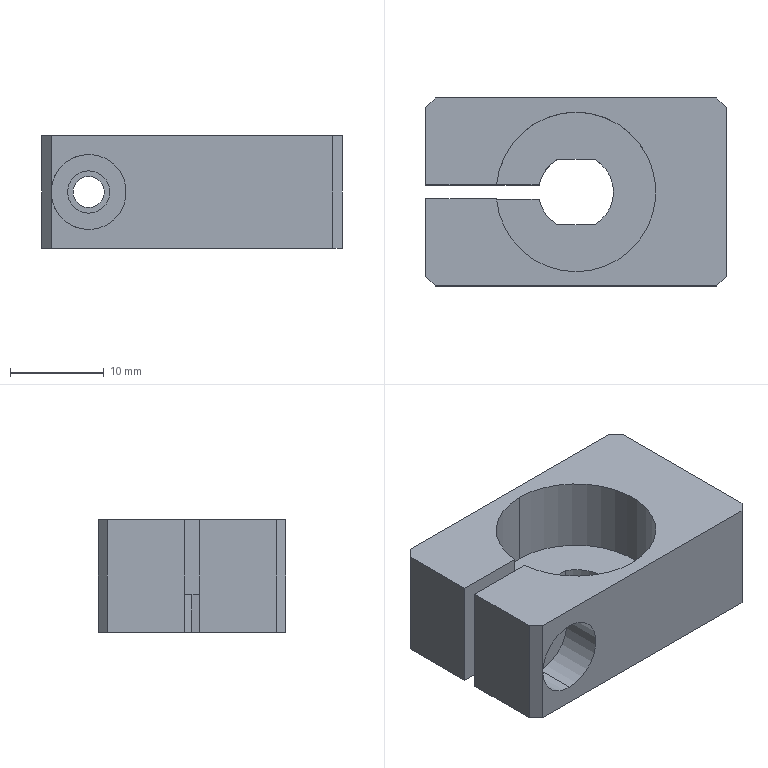Part | SolidWorks | features ICE 3, HoleWzd 2, Chamfer 1, Extrusion 1, RevCut 1 | 1 solid | 30 faces | box 32 x 20 x 12 mm | volume 5110 mm3 | plane 17 | cylinder 13 | commonest cylinder face diameters 8 x6 17 x3 3.3 x2 4.5 x2
STEP:
#1=CARTESIAN_POINT('',(-11.,10.,1.65));
#2=VERTEX_POINT('',#1);
#3=CARTESIAN_POINT('',(-11.,10.,-1.65));
#4=VERTEX_POINT('',#3);
#5=CARTESIAN_POINT('',(-11.,10.,0.));
#6=DIRECTION('',(0.,-1.,0.));
#7=DIRECTION('',(0.,0.,-1.));
#8=AXIS2_PLACEMENT_3D('',#5,#6,#7);
#9=CIRCLE('',#8,1.65);
#10=EDGE_CURVE('',#2,#4,#9,.T.);
#11=ORIENTED_EDGE('',*,*,#10,.F.);
#12=CARTESIAN_POINT('',(-11.,0.75,1.65));
#13=VERTEX_POINT('',#12);
#14=CARTESIAN_POINT('',(-11.,0.75,1.65));
#15=DIRECTION('',(0.,-1.,0.));
#16=VECTOR('',#15,1000.);
#17=LINE('',#14,#16);
#18=EDGE_CURVE('',#2,#13,#17,.T.);
#19=ORIENTED_EDGE('',*,*,#18,.T.);
#20=CARTESIAN_POINT('',(-11.,0.75,-1.65));
#21=VERTEX_POINT('',#20);
#22=CARTESIAN_POINT('',(-11.,0.75,0.));
#23=DIRECTION('',(0.,-1.,0.));
#24=DIRECTION('',(0.,0.,-1.));
#25=AXIS2_PLACEMENT_3D('',#22,#23,#24);
#26=CIRCLE('',#25,1.65);
#27=EDGE_CURVE('',#13,#21,#26,.T.);
#28=ORIENTED_EDGE('',*,*,#27,.T.);
#29=CARTESIAN_POINT('',(-11.,0.75,-1.65));
#30=DIRECTION('',(0.,-1.,0.));
#31=VECTOR('',#30,1000.);
#32=LINE('',#29,#31);
#33=EDGE_CURVE('',#4,#21,#32,.T.);
#34=ORIENTED_EDGE('',*,*,#33,.F.);
#35=EDGE_LOOP('',(#11,#19,#28,#34));
#36=FACE_OUTER_BOUND('',#35,.T.);
#37=CARTESIAN_POINT('',(-11.,0.75,0.));
#38=DIRECTION('',(0.,-1.,0.));
#39=DIRECTION('',(0.,0.,-1.));
#40=AXIS2_PLACEMENT_3D('',#37,#38,#39);
#41=CYLINDRICAL_SURFACE('',#40,1.65);
#42=ADVANCED_FACE('',(#36),#41,.F.);
#43=CARTESIAN_POINT('',(-11.,-5.6,4.));
#44=VERTEX_POINT('',#43);
#45=CARTESIAN_POINT('',(-11.,-5.6,-4.));
#46=VERTEX_POINT('',#45);
#47=CARTESIAN_POINT('',(-11.,-5.6,0.));
#48=DIRECTION('',(0.,-1.,0.));
#49=DIRECTION('',(0.,0.,-1.));
#50=AXIS2_PLACEMENT_3D('',#47,#48,#49);
#51=CIRCLE('',#50,4.);
#52=EDGE_CURVE('',#44,#46,#51,.T.);
#53=ORIENTED_EDGE('',*,*,#52,.F.);
#54=CARTESIAN_POINT('',(-11.,-10.,4.));
#55=VERTEX_POINT('',#54);
#56=CARTESIAN_POINT('',(-11.,-10.,4.));
#57=DIRECTION('',(0.,-1.,0.));
#58=VECTOR('',#57,1000.);
#59=LINE('',#56,#58);
#60=EDGE_CURVE('',#44,#55,#59,.T.);
#61=ORIENTED_EDGE('',*,*,#60,.T.);
#62=CARTESIAN_POINT('',(-15.,-10.,0.));
#63=VERTEX_POINT('',#62);
#64=CARTESIAN_POINT('',(-11.,-10.,0.));
#65=DIRECTION('',(0.,-1.,0.));
#66=DIRECTION('',(0.,0.,-1.));
#67=AXIS2_PLACEMENT_3D('',#64,#65,#66);
#68=CIRCLE('',#67,4.);
#69=EDGE_CURVE('',#55,#63,#68,.T.);
#70=ORIENTED_EDGE('',*,*,#69,.T.);
#71=CARTESIAN_POINT('',(-11.,-10.,-4.));
#72=VERTEX_POINT('',#71);
#73=CARTESIAN_POINT('',(-11.,-10.,0.));
#74=DIRECTION('',(0.,-1.,0.));
#75=DIRECTION('',(0.,0.,-1.));
#76=AXIS2_PLACEMENT_3D('',#73,#74,#75);
#77=CIRCLE('',#76,4.);
#78=EDGE_CURVE('',#63,#72,#77,.T.);
#79=ORIENTED_EDGE('',*,*,#78,.T.);
#80=CARTESIAN_POINT('',(-11.,-10.,-4.));
#81=DIRECTION('',(0.,-1.,0.));
#82=VECTOR('',#81,1000.);
#83=LINE('',#80,#82);
#84=EDGE_CURVE('',#46,#72,#83,.T.);
#85=ORIENTED_EDGE('',*,*,#84,.F.);
#86=EDGE_LOOP('',(#53,#61,#70,#79,#85));
#87=FACE_OUTER_BOUND('',#86,.T.);
#88=CARTESIAN_POINT('',(-11.,-10.,0.));
#89=DIRECTION('',(0.,-1.,0.));
#90=DIRECTION('',(0.,0.,-1.));
#91=AXIS2_PLACEMENT_3D('',#88,#89,#90);
#92=CYLINDRICAL_SURFACE('',#91,4.);
#93=ADVANCED_FACE('',(#87),#92,.F.);
#94=CARTESIAN_POINT('',(-11.,-0.75,2.25));
#95=VERTEX_POINT('',#94);
#96=CARTESIAN_POINT('',(-11.,-0.75,-2.25));
#97=VERTEX_POINT('',#96);
#98=CARTESIAN_POINT('',(-11.,-0.75,0.));
#99=DIRECTION('',(0.,-1.,0.));
#100=DIRECTION('',(0.,0.,-1.));
#101=AXIS2_PLACEMENT_3D('',#98,#99,#100);
#102=CIRCLE('',#101,2.25);
#103=EDGE_CURVE('',#95,#97,#102,.T.);
#104=ORIENTED_EDGE('',*,*,#103,.F.);
#105=CARTESIAN_POINT('',(-11.,-5.6,2.25));
#106=VERTEX_POINT('',#105);
#107=CARTESIAN_POINT('',(-11.,-10.,2.25));
#108=DIRECTION('',(0.,-1.,0.));
#109=VECTOR('',#108,1000.);
#110=LINE('',#107,#109);
#111=EDGE_CURVE('',#95,#106,#110,.T.);
#112=ORIENTED_EDGE('',*,*,#111,.T.);
#113=CARTESIAN_POINT('',(-11.,-5.6,-2.25));
#114=VERTEX_POINT('',#113);
#115=CARTESIAN_POINT('',(-11.,-5.6,0.));
#116=DIRECTION('',(0.,-1.,0.));
#117=DIRECTION('',(0.,0.,-1.));
#118=AXIS2_PLACEMENT_3D('',#115,#116,#117);
#119=CIRCLE('',#118,2.25);
#120=EDGE_CURVE('',#106,#114,#119,.T.);
#121=ORIENTED_EDGE('',*,*,#120,.T.);
#122=CARTESIAN_POINT('',(-11.,-10.,-2.25));
#123=DIRECTION('',(0.,-1.,0.));
#124=VECTOR('',#123,1000.);
#125=LINE('',#122,#124);
#126=EDGE_CURVE('',#97,#114,#125,.T.);
#127=ORIENTED_EDGE('',*,*,#126,.F.);
#128=EDGE_LOOP('',(#104,#112,#121,#127));
#129=FACE_OUTER_BOUND('',#128,.T.);
#130=CARTESIAN_POINT('',(-11.,-10.,0.));
#131=DIRECTION('',(0.,-1.,0.));
#132=DIRECTION('',(0.,0.,-1.));
#133=AXIS2_PLACEMENT_3D('',#130,#131,#132);
#134=CYLINDRICAL_SURFACE('',#133,2.25);
#135=ADVANCED_FACE('',(#129),#134,.F.);
#136=CARTESIAN_POINT('',(0.,-8.5,6.));
#137=VERTEX_POINT('',#136);
#138=CARTESIAN_POINT('',(-8.467,-0.75,6.));
#139=VERTEX_POINT('',#138);
#140=CARTESIAN_POINT('',(0.,0.,6.));
#141=DIRECTION('',(0.,0.,-1.));
#142=DIRECTION('',(0.,1.,0.));
#143=AXIS2_PLACEMENT_3D('',#140,#141,#142);
#144=CIRCLE('',#143,8.5);
#145=EDGE_CURVE('',#137,#139,#144,.T.);
#146=ORIENTED_EDGE('',*,*,#145,.F.);
#147=CARTESIAN_POINT('',(0.,-8.5,-2.));
#148=VERTEX_POINT('',#147);
#149=CARTESIAN_POINT('',(0.,-8.5,-2.));
#150=DIRECTION('',(0.,0.,-1.));
#151=VECTOR('',#150,1000.);
#152=LINE('',#149,#151);
#153=EDGE_CURVE('',#137,#148,#152,.T.);
#154=ORIENTED_EDGE('',*,*,#153,.T.);
#155=CARTESIAN_POINT('',(-8.467,-0.75,-2.));
#156=VERTEX_POINT('',#155);
#157=CARTESIAN_POINT('',(0.,0.,-2.));
#158=DIRECTION('',(0.,0.,-1.));
#159=DIRECTION('',(0.,1.,0.));
#160=AXIS2_PLACEMENT_3D('',#157,#158,#159);
#161=CIRCLE('',#160,8.5);
#162=EDGE_CURVE('',#148,#156,#161,.T.);
#163=ORIENTED_EDGE('',*,*,#162,.T.);
#164=CARTESIAN_POINT('',(-8.467,-0.75,-2.));
#165=DIRECTION('',(0.,0.,1.));
#166=VECTOR('',#165,1000.);
#167=LINE('',#164,#166);
#168=EDGE_CURVE('',#156,#139,#167,.T.);
#169=ORIENTED_EDGE('',*,*,#168,.T.);
#170=EDGE_LOOP('',(#146,#154,#163,#169));
#171=FACE_OUTER_BOUND('',#170,.T.);
#172=CARTESIAN_POINT('',(0.,0.,-2.));
#173=DIRECTION('',(0.,0.,-1.));
#174=DIRECTION('',(0.,1.,0.));
#175=AXIS2_PLACEMENT_3D('',#172,#173,#174);
#176=CYLINDRICAL_SURFACE('',#175,8.5);
#177=ADVANCED_FACE('',(#171),#176,.F.);
#178=ORIENTED_EDGE('',*,*,#153,.F.);
#179=CARTESIAN_POINT('',(0.,8.5,6.));
#180=VERTEX_POINT('',#179);
#181=CARTESIAN_POINT('',(0.,0.,6.));
#182=DIRECTION('',(0.,0.,-1.));
#183=DIRECTION('',(0.,1.,0.));
#184=AXIS2_PLACEMENT_3D('',#181,#182,#183);
#185=CIRCLE('',#184,8.5);
#186=EDGE_CURVE('',#180,#137,#185,.T.);
#187=ORIENTED_EDGE('',*,*,#186,.F.);
#188=CARTESIAN_POINT('',(0.,8.5,-2.));
#189=VERTEX_POINT('',#188);
#190=CARTESIAN_POINT('',(0.,8.5,-2.));
#191=DIRECTION('',(0.,0.,-1.));
#192=VECTOR('',#191,1000.);
#193=LINE('',#190,#192);
#194=EDGE_CURVE('',#180,#189,#193,.T.);
#195=ORIENTED_EDGE('',*,*,#194,.T.);
#196=CARTESIAN_POINT('',(0.,0.,-2.));
#197=DIRECTION('',(0.,0.,-1.));
#198=DIRECTION('',(0.,1.,0.));
#199=AXIS2_PLACEMENT_3D('',#196,#197,#198);
#200=CIRCLE('',#199,8.5);
#201=EDGE_CURVE('',#189,#148,#200,.T.);
#202=ORIENTED_EDGE('',*,*,#201,.T.);
#203=EDGE_LOOP('',(#178,#187,#195,#202));
#204=FACE_OUTER_BOUND('',#203,.T.);
#205=CARTESIAN_POINT('',(0.,0.,-2.));
#206=DIRECTION('',(0.,0.,-1.));
#207=DIRECTION('',(0.,1.,0.));
#208=AXIS2_PLACEMENT_3D('',#205,#206,#207);
#209=CYLINDRICAL_SURFACE('',#208,8.5);
#210=ADVANCED_FACE('',(#204),#209,.F.);
#211=CARTESIAN_POINT('',(4.,0.,-6.));
#212=VERTEX_POINT('',#211);
#213=CARTESIAN_POINT('',(1.936,3.5,-6.));
#214=VERTEX_POINT('',#213);
#215=CARTESIAN_POINT('',(0.,0.,-6.));
#216=DIRECTION('',(0.,0.,1.));
#217=DIRECTION('',(1.,0.,0.));
#218=AXIS2_PLACEMENT_3D('',#215,#216,#217);
#219=CIRCLE('',#218,4.);
#220=EDGE_CURVE('',#212,#214,#219,.T.);
#221=ORIENTED_EDGE('',*,*,#220,.F.);
#222=CARTESIAN_POINT('',(4.,0.,-2.));
#223=VERTEX_POINT('',#222);
#224=CARTESIAN_POINT('',(4.,0.,-6.));
#225=DIRECTION('',(0.,0.,1.));
#226=VECTOR('',#225,1000.);
#227=LINE('',#224,#226);
#228=EDGE_CURVE('',#212,#223,#227,.T.);
#229=ORIENTED_EDGE('',*,*,#228,.T.);
#230=CARTESIAN_POINT('',(1.936,3.5,-2.));
#231=VERTEX_POINT('',#230);
#232=CARTESIAN_POINT('',(0.,0.,-2.));
#233=DIRECTION('',(0.,0.,1.));
#234=DIRECTION('',(0.,1.,0.));
#235=AXIS2_PLACEMENT_3D('',#232,#233,#234);
#236=CIRCLE('',#235,4.);
#237=EDGE_CURVE('',#223,#231,#236,.T.);
#238=ORIENTED_EDGE('',*,*,#237,.T.);
#239=CARTESIAN_POINT('',(1.936,3.5,-2.));
#240=DIRECTION('',(0.,0.,-1.));
#241=VECTOR('',#240,1000.);
#242=LINE('',#239,#241);
#243=EDGE_CURVE('',#231,#214,#242,.T.);
#244=ORIENTED_EDGE('',*,*,#243,.T.);
#245=EDGE_LOOP('',(#221,#229,#238,#244));
#246=FACE_OUTER_BOUND('',#245,.T.);
#247=CARTESIAN_POINT('',(0.,0.,-6.));
#248=DIRECTION('',(0.,0.,1.));
#249=DIRECTION('',(1.,0.,0.));
#250=AXIS2_PLACEMENT_3D('',#247,#248,#249);
#251=CYLINDRICAL_SURFACE('',#250,4.);
#252=ADVANCED_FACE('',(#246),#251,.F.);
#253=CARTESIAN_POINT('',(-15.,-10.,-6.));
#254=VERTEX_POINT('',#253);
#255=CARTESIAN_POINT('',(15.,-10.,-6.));
#256=VERTEX_POINT('',#255);
#257=CARTESIAN_POINT('',(-16.,-10.,-6.));
#258=DIRECTION('',(1.,0.,0.));
#259=VECTOR('',#258,1000.);
#260=LINE('',#257,#259);
#261=EDGE_CURVE('',#254,#256,#260,.T.);
#262=ORIENTED_EDGE('',*,*,#261,.T.);
#263=CARTESIAN_POINT('',(15.,-10.,6.));
#264=VERTEX_POINT('',#263);
#265=CARTESIAN_POINT('',(15.,-10.,6.));
#266=DIRECTION('',(0.,0.,1.));
#267=VECTOR('',#266,1000.);
#268=LINE('',#265,#267);
#269=EDGE_CURVE('',#256,#264,#268,.T.);
#270=ORIENTED_EDGE('',*,*,#269,.T.);
#271=CARTESIAN_POINT('',(-15.,-10.,6.));
#272=VERTEX_POINT('',#271);
#273=CARTESIAN_POINT('',(-16.,-10.,6.));
#274=DIRECTION('',(1.,0.,0.));
#275=VECTOR('',#274,1000.);
#276=LINE('',#273,#275);
#277=EDGE_CURVE('',#272,#264,#276,.T.);
#278=ORIENTED_EDGE('',*,*,#277,.F.);
#279=CARTESIAN_POINT('',(-15.,-10.,6.));
#280=DIRECTION('',(0.,0.,-1.));
#281=VECTOR('',#280,1000.);
#282=LINE('',#279,#281);
#283=EDGE_CURVE('',#272,#63,#282,.T.);
#284=ORIENTED_EDGE('',*,*,#283,.T.);
#285=ORIENTED_EDGE('',*,*,#69,.F.);
#286=CARTESIAN_POINT('',(-11.,-10.,0.));
#287=DIRECTION('',(0.,-1.,0.));
#288=DIRECTION('',(0.,0.,-1.));
#289=AXIS2_PLACEMENT_3D('',#286,#287,#288);
#290=CIRCLE('',#289,4.);
#291=EDGE_CURVE('',#72,#55,#290,.T.);
#292=ORIENTED_EDGE('',*,*,#291,.F.);
#293=ORIENTED_EDGE('',*,*,#78,.F.);
#294=CARTESIAN_POINT('',(-15.,-10.,6.));
#295=DIRECTION('',(0.,0.,-1.));
#296=VECTOR('',#295,1000.);
#297=LINE('',#294,#296);
#298=EDGE_CURVE('',#63,#254,#297,.T.);
#299=ORIENTED_EDGE('',*,*,#298,.T.);
#300=EDGE_LOOP('',(#262,#270,#278,#284,#285,#292,#293,#299));
#301=FACE_OUTER_BOUND('',#300,.T.);
#302=CARTESIAN_POINT('',(-16.,-10.,6.));
#303=DIRECTION('',(0.,1.,0.));
#304=DIRECTION('',(0.,0.,1.));
#305=AXIS2_PLACEMENT_3D('',#302,#303,#304);
#306=PLANE('',#305);
#307=ADVANCED_FACE('',(#301),#306,.F.);
#308=CARTESIAN_POINT('',(-16.,9.,6.));
#309=VERTEX_POINT('',#308);
#310=CARTESIAN_POINT('',(-16.,0.75,6.));
#311=VERTEX_POINT('',#310);
#312=CARTESIAN_POINT('',(-16.,10.,6.));
#313=DIRECTION('',(0.,-1.,0.));
#314=VECTOR('',#313,1000.);
#315=LINE('',#312,#314);
#316=EDGE_CURVE('',#309,#311,#315,.T.);
#317=ORIENTED_EDGE('',*,*,#316,.F.);
#318=CARTESIAN_POINT('',(-16.,9.,-6.));
#319=VERTEX_POINT('',#318);
#320=CARTESIAN_POINT('',(-16.,9.,6.));
#321=DIRECTION('',(0.,0.,-1.));
#322=VECTOR('',#321,1000.);
#323=LINE('',#320,#322);
#324=EDGE_CURVE('',#309,#319,#323,.T.);
#325=ORIENTED_EDGE('',*,*,#324,.T.);
#326=CARTESIAN_POINT('',(-16.,0.75,-6.));
#327=VERTEX_POINT('',#326);
#328=CARTESIAN_POINT('',(-16.,10.,-6.));
#329=DIRECTION('',(0.,-1.,0.));
#330=VECTOR('',#329,1000.);
#331=LINE('',#328,#330);
#332=EDGE_CURVE('',#319,#327,#331,.T.);
#333=ORIENTED_EDGE('',*,*,#332,.T.);
#334=CARTESIAN_POINT('',(-16.,0.75,6.));
#335=DIRECTION('',(0.,0.,1.));
#336=VECTOR('',#335,1000.);
#337=LINE('',#334,#336);
#338=EDGE_CURVE('',#327,#311,#337,.T.);
#339=ORIENTED_EDGE('',*,*,#338,.T.);
#340=EDGE_LOOP('',(#317,#325,#333,#339));
#341=FACE_OUTER_BOUND('',#340,.T.);
#342=CARTESIAN_POINT('',(-16.,10.,6.));
#343=DIRECTION('',(1.,0.,0.));
#344=DIRECTION('',(0.,1.,0.));
#345=AXIS2_PLACEMENT_3D('',#342,#343,#344);
#346=PLANE('',#345);
#347=ADVANCED_FACE('',(#341),#346,.F.);
#348=CARTESIAN_POINT('',(-1.936,3.5,-2.));
#349=VERTEX_POINT('',#348);
#350=CARTESIAN_POINT('',(-3.929,0.75,-2.));
#351=VERTEX_POINT('',#350);
#352=CARTESIAN_POINT('',(0.,0.,-2.));
#353=DIRECTION('',(0.,0.,1.));
#354=DIRECTION('',(0.,1.,0.));
#355=AXIS2_PLACEMENT_3D('',#352,#353,#354);
#356=CIRCLE('',#355,4.);
#357=EDGE_CURVE('',#349,#351,#356,.T.);
#358=ORIENTED_EDGE('',*,*,#357,.T.);
#359=CARTESIAN_POINT('',(-3.929,0.75,-6.));
#360=VERTEX_POINT('',#359);
#361=CARTESIAN_POINT('',(-3.929,0.75,-6.));
#362=DIRECTION('',(0.,0.,-1.));
#363=VECTOR('',#362,1000.);
#364=LINE('',#361,#363);
#365=EDGE_CURVE('',#351,#360,#364,.T.);
#366=ORIENTED_EDGE('',*,*,#365,.T.);
#367=CARTESIAN_POINT('',(-1.936,3.5,-6.));
#368=VERTEX_POINT('',#367);
#369=CARTESIAN_POINT('',(0.,0.,-6.));
#370=DIRECTION('',(0.,0.,1.));
#371=DIRECTION('',(1.,0.,0.));
#372=AXIS2_PLACEMENT_3D('',#369,#370,#371);
#373=CIRCLE('',#372,4.);
#374=EDGE_CURVE('',#368,#360,#373,.T.);
#375=ORIENTED_EDGE('',*,*,#374,.F.);
#376=CARTESIAN_POINT('',(-1.936,3.5,-2.));
#377=DIRECTION('',(0.,0.,-1.));
#378=VECTOR('',#377,1000.);
#379=LINE('',#376,#378);
#380=EDGE_CURVE('',#349,#368,#379,.T.);
#381=ORIENTED_EDGE('',*,*,#380,.F.);
#382=EDGE_LOOP('',(#358,#366,#375,#381));
#383=FACE_OUTER_BOUND('',#382,.T.);
#384=CARTESIAN_POINT('',(0.,0.,-6.));
#385=DIRECTION('',(0.,0.,1.));
#386=DIRECTION('',(1.,0.,0.));
#387=AXIS2_PLACEMENT_3D('',#384,#385,#386);
#388=CYLINDRICAL_SURFACE('',#387,4.);
#389=ADVANCED_FACE('',(#383),#388,.F.);
#390=ORIENTED_EDGE('',*,*,#228,.F.);
#391=CARTESIAN_POINT('',(1.936,-3.5,-6.));
#392=VERTEX_POINT('',#391);
#393=CARTESIAN_POINT('',(0.,0.,-6.));
#394=DIRECTION('',(0.,0.,1.));
#395=DIRECTION('',(1.,0.,0.));
#396=AXIS2_PLACEMENT_3D('',#393,#394,#395);
#397=CIRCLE('',#396,4.);
#398=EDGE_CURVE('',#392,#212,#397,.T.);
#399=ORIENTED_EDGE('',*,*,#398,.F.);
#400=CARTESIAN_POINT('',(1.936,-3.5,-2.));
#401=VERTEX_POINT('',#400);
#402=CARTESIAN_POINT('',(1.936,-3.5,-2.));
#403=DIRECTION('',(0.,0.,-1.));
#404=VECTOR('',#403,1000.);
#405=LINE('',#402,#404);
#406=EDGE_CURVE('',#401,#392,#405,.T.);
#407=ORIENTED_EDGE('',*,*,#406,.F.);
#408=CARTESIAN_POINT('',(0.,0.,-2.));
#409=DIRECTION('',(0.,0.,1.));
#410=DIRECTION('',(0.,1.,0.));
#411=AXIS2_PLACEMENT_3D('',#408,#409,#410);
#412=CIRCLE('',#411,4.);
#413=EDGE_CURVE('',#401,#223,#412,.T.);
#414=ORIENTED_EDGE('',*,*,#413,.T.);
#415=EDGE_LOOP('',(#390,#399,#407,#414));
#416=FACE_OUTER_BOUND('',#415,.T.);
#417=CARTESIAN_POINT('',(0.,0.,-6.));
#418=DIRECTION('',(0.,0.,1.));
#419=DIRECTION('',(1.,0.,0.));
#420=AXIS2_PLACEMENT_3D('',#417,#418,#419);
#421=CYLINDRICAL_SURFACE('',#420,4.);
#422=ADVANCED_FACE('',(#416),#421,.F.);
#423=CARTESIAN_POINT('',(16.,-9.,-6.));
#424=VERTEX_POINT('',#423);
#425=CARTESIAN_POINT('',(16.,9.,-6.));
#426=VERTEX_POINT('',#425);
#427=CARTESIAN_POINT('',(16.,10.,-6.));
#428=DIRECTION('',(0.,1.,0.));
#429=VECTOR('',#428,1000.);
#430=LINE('',#427,#429);
#431=EDGE_CURVE('',#424,#426,#430,.T.);
#432=ORIENTED_EDGE('',*,*,#431,.T.);
#433=CARTESIAN_POINT('',(16.,9.,6.));
#434=VERTEX_POINT('',#433);
#435=CARTESIAN_POINT('',(16.,9.,6.));
#436=DIRECTION('',(0.,0.,1.));
#437=VECTOR('',#436,1000.);
#438=LINE('',#435,#437);
#439=EDGE_CURVE('',#426,#434,#438,.T.);
#440=ORIENTED_EDGE('',*,*,#439,.T.);
#441=CARTESIAN_POINT('',(16.,-9.,6.));
#442=VERTEX_POINT('',#441);
#443=CARTESIAN_POINT('',(16.,10.,6.));
#444=DIRECTION('',(0.,1.,0.));
#445=VECTOR('',#444,1000.);
#446=LINE('',#443,#445);
#447=EDGE_CURVE('',#442,#434,#446,.T.);
#448=ORIENTED_EDGE('',*,*,#447,.F.);
#449=CARTESIAN_POINT('',(16.,-9.,6.));
#450=DIRECTION('',(0.,0.,-1.));
#451=VECTOR('',#450,1000.);
#452=LINE('',#449,#451);
#453=EDGE_CURVE('',#442,#424,#452,.T.);
#454=ORIENTED_EDGE('',*,*,#453,.T.);
#455=EDGE_LOOP('',(#432,#440,#448,#454));
#456=FACE_OUTER_BOUND('',#455,.T.);
#457=CARTESIAN_POINT('',(16.,10.,6.));
#458=DIRECTION('',(-1.,0.,0.));
#459=DIRECTION('',(0.,-1.,0.));
#460=AXIS2_PLACEMENT_3D('',#457,#458,#459);
#461=PLANE('',#460);
#462=ADVANCED_FACE('',(#456),#461,.F.);
#463=CARTESIAN_POINT('',(-11.,10.,0.));
#464=DIRECTION('',(0.,-1.,0.));
#465=DIRECTION('',(0.,0.,-1.));
#466=AXIS2_PLACEMENT_3D('',#463,#464,#465);
#467=CIRCLE('',#466,1.65);
#468=EDGE_CURVE('',#4,#2,#467,.T.);
#469=ORIENTED_EDGE('',*,*,#468,.T.);
#470=ORIENTED_EDGE('',*,*,#10,.T.);
#471=EDGE_LOOP('',(#469,#470));
#472=FACE_BOUND('',#471,.T.);
#473=CARTESIAN_POINT('',(15.,10.,6.));
#474=VERTEX_POINT('',#473);
#475=CARTESIAN_POINT('',(-15.,10.,6.));
#476=VERTEX_POINT('',#475);
#477=CARTESIAN_POINT('',(-16.,10.,6.));
#478=DIRECTION('',(-1.,0.,0.));
#479=VECTOR('',#478,1000.);
#480=LINE('',#477,#479);
#481=EDGE_CURVE('',#474,#476,#480,.T.);
#482=ORIENTED_EDGE('',*,*,#481,.F.);
#483=CARTESIAN_POINT('',(15.,10.,-6.));
#484=VERTEX_POINT('',#483);
#485=CARTESIAN_POINT('',(15.,10.,6.));
#486=DIRECTION('',(0.,0.,-1.));
#487=VECTOR('',#486,1000.);
#488=LINE('',#485,#487);
#489=EDGE_CURVE('',#474,#484,#488,.T.);
#490=ORIENTED_EDGE('',*,*,#489,.T.);
#491=CARTESIAN_POINT('',(-15.,10.,-6.));
#492=VERTEX_POINT('',#491);
#493=CARTESIAN_POINT('',(-16.,10.,-6.));
#494=DIRECTION('',(-1.,0.,0.));
#495=VECTOR('',#494,1000.);
#496=LINE('',#493,#495);
#497=EDGE_CURVE('',#484,#492,#496,.T.);
#498=ORIENTED_EDGE('',*,*,#497,.T.);
#499=CARTESIAN_POINT('',(-15.,10.,6.));
#500=DIRECTION('',(0.,0.,1.));
#501=VECTOR('',#500,1000.);
#502=LINE('',#499,#501);
#503=EDGE_CURVE('',#492,#476,#502,.T.);
#504=ORIENTED_EDGE('',*,*,#503,.T.);
#505=EDGE_LOOP('',(#482,#490,#498,#504));
#506=FACE_OUTER_BOUND('',#505,.T.);
#507=CARTESIAN_POINT('',(-16.,10.,6.));
#508=DIRECTION('',(0.,-1.,0.));
#509=DIRECTION('',(0.,0.,-1.));
#510=AXIS2_PLACEMENT_3D('',#507,#508,#509);
#511=PLANE('',#510);
#512=ADVANCED_FACE('',(#472,#506),#511,.F.);
#513=CARTESIAN_POINT('',(-16.,-0.75,-6.));
#514=VERTEX_POINT('',#513);
#515=CARTESIAN_POINT('',(-16.,-9.,-6.));
#516=VERTEX_POINT('',#515);
#517=CARTESIAN_POINT('',(-16.,10.,-6.));
#518=DIRECTION('',(0.,-1.,0.));
#519=VECTOR('',#518,1000.);
#520=LINE('',#517,#519);
#521=EDGE_CURVE('',#514,#516,#520,.T.);
#522=ORIENTED_EDGE('',*,*,#521,.T.);
#523=CARTESIAN_POINT('',(-16.,-9.,6.));
#524=VERTEX_POINT('',#523);
#525=CARTESIAN_POINT('',(-16.,-9.,6.));
#526=DIRECTION('',(0.,0.,1.));
#527=VECTOR('',#526,1000.);
#528=LINE('',#525,#527);
#529=EDGE_CURVE('',#516,#524,#528,.T.);
#530=ORIENTED_EDGE('',*,*,#529,.T.);
#531=CARTESIAN_POINT('',(-16.,-0.75,6.));
#532=VERTEX_POINT('',#531);
#533=CARTESIAN_POINT('',(-16.,10.,6.));
#534=DIRECTION('',(0.,-1.,0.));
#535=VECTOR('',#534,1000.);
#536=LINE('',#533,#535);
#537=EDGE_CURVE('',#532,#524,#536,.T.);
#538=ORIENTED_EDGE('',*,*,#537,.F.);
#539=CARTESIAN_POINT('',(-16.,-0.75,6.));
#540=DIRECTION('',(0.,0.,-1.));
#541=VECTOR('',#540,1000.);
#542=LINE('',#539,#541);
#543=EDGE_CURVE('',#532,#514,#542,.T.);
#544=ORIENTED_EDGE('',*,*,#543,.T.);
#545=EDGE_LOOP('',(#522,#530,#538,#544));
#546=FACE_OUTER_BOUND('',#545,.T.);
#547=CARTESIAN_POINT('',(-16.,10.,6.));
#548=DIRECTION('',(1.,0.,0.));
#549=DIRECTION('',(0.,1.,0.));
#550=AXIS2_PLACEMENT_3D('',#547,#548,#549);
#551=PLANE('',#550);
#552=ADVANCED_FACE('',(#546),#551,.F.);
#553=ORIENTED_EDGE('',*,*,#447,.T.);
#554=CARTESIAN_POINT('',(12.5,12.5,6.));
#555=DIRECTION('',(-0.7071,0.7071,0.));
#556=VECTOR('',#555,1000.);
#557=LINE('',#554,#556);
#558=EDGE_CURVE('',#434,#474,#557,.T.);
#559=ORIENTED_EDGE('',*,*,#558,.T.);
#560=ORIENTED_EDGE('',*,*,#481,.T.);
#561=CARTESIAN_POINT('',(-12.5,12.5,6.));
#562=DIRECTION('',(-0.7071,-0.7071,0.));
#563=VECTOR('',#562,1000.);
#564=LINE('',#561,#563);
#565=EDGE_CURVE('',#476,#309,#564,.T.);
#566=ORIENTED_EDGE('',*,*,#565,.T.);
#567=ORIENTED_EDGE('',*,*,#316,.T.);
#568=CARTESIAN_POINT('',(-8.467,0.75,6.));
#569=VERTEX_POINT('',#568);
#570=CARTESIAN_POINT('',(1.63,0.75,6.));
#571=DIRECTION('',(1.,0.,0.));
#572=VECTOR('',#571,1000.);
#573=LINE('',#570,#572);
#574=EDGE_CURVE('',#311,#569,#573,.T.);
#575=ORIENTED_EDGE('',*,*,#574,.T.);
#576=CARTESIAN_POINT('',(0.,0.,6.));
#577=DIRECTION('',(0.,0.,-1.));
#578=DIRECTION('',(0.,1.,0.));
#579=AXIS2_PLACEMENT_3D('',#576,#577,#578);
#580=CIRCLE('',#579,8.5);
#581=EDGE_CURVE('',#569,#180,#580,.T.);
#582=ORIENTED_EDGE('',*,*,#581,.T.);
#583=ORIENTED_EDGE('',*,*,#186,.T.);
#584=ORIENTED_EDGE('',*,*,#145,.T.);
#585=CARTESIAN_POINT('',(1.63,-0.75,6.));
#586=DIRECTION('',(-1.,0.,0.));
#587=VECTOR('',#586,1000.);
#588=LINE('',#585,#587);
#589=EDGE_CURVE('',#139,#532,#588,.T.);
#590=ORIENTED_EDGE('',*,*,#589,.T.);
#591=ORIENTED_EDGE('',*,*,#537,.T.);
#592=CARTESIAN_POINT('',(-12.5,-12.5,6.));
#593=DIRECTION('',(0.7071,-0.7071,0.));
#594=VECTOR('',#593,1000.);
#595=LINE('',#592,#594);
#596=EDGE_CURVE('',#524,#272,#595,.T.);
#597=ORIENTED_EDGE('',*,*,#596,.T.);
#598=ORIENTED_EDGE('',*,*,#277,.T.);
#599=CARTESIAN_POINT('',(12.5,-12.5,6.));
#600=DIRECTION('',(0.7071,0.7071,0.));
#601=VECTOR('',#600,1000.);
#602=LINE('',#599,#601);
#603=EDGE_CURVE('',#264,#442,#602,.T.);
#604=ORIENTED_EDGE('',*,*,#603,.T.);
#605=EDGE_LOOP('',(#553,#559,#560,#566,#567,#575,#582,#583,#584,#590,#591,#597,#598,#604));
#606=FACE_OUTER_BOUND('',#605,.T.);
#607=CARTESIAN_POINT('',(0.,0.,6.));
#608=DIRECTION('',(0.,0.,1.));
#609=DIRECTION('',(1.,0.,0.));
#610=AXIS2_PLACEMENT_3D('',#607,#608,#609);
#611=PLANE('',#610);
#612=ADVANCED_FACE('',(#606),#611,.T.);
#613=ORIENTED_EDGE('',*,*,#497,.F.);
#614=CARTESIAN_POINT('',(15.,10.,-6.));
#615=DIRECTION('',(0.7071,-0.7071,0.));
#616=VECTOR('',#615,1000.);
#617=LINE('',#614,#616);
#618=EDGE_CURVE('',#484,#426,#617,.T.);
#619=ORIENTED_EDGE('',*,*,#618,.T.);
#620=ORIENTED_EDGE('',*,*,#431,.F.);
#621=CARTESIAN_POINT('',(16.,-9.,-6.));
#622=DIRECTION('',(-0.7071,-0.7071,0.));
#623=VECTOR('',#622,1000.);
#624=LINE('',#621,#623);
#625=EDGE_CURVE('',#424,#256,#624,.T.);
#626=ORIENTED_EDGE('',*,*,#625,.T.);
#627=ORIENTED_EDGE('',*,*,#261,.F.);
#628=CARTESIAN_POINT('',(-15.,-10.,-6.));
#629=DIRECTION('',(-0.7071,0.7071,0.));
#630=VECTOR('',#629,1000.);
#631=LINE('',#628,#630);
#632=EDGE_CURVE('',#254,#516,#631,.T.);
#633=ORIENTED_EDGE('',*,*,#632,.T.);
#634=ORIENTED_EDGE('',*,*,#521,.F.);
#635=CARTESIAN_POINT('',(-3.929,-0.75,-6.));
#636=VERTEX_POINT('',#635);
#637=CARTESIAN_POINT('',(1.63,-0.75,-6.));
#638=DIRECTION('',(-1.,0.,0.));
#639=VECTOR('',#638,1000.);
#640=LINE('',#637,#639);
#641=EDGE_CURVE('',#636,#514,#640,.T.);
#642=ORIENTED_EDGE('',*,*,#641,.F.);
#643=CARTESIAN_POINT('',(-1.936,-3.5,-6.));
#644=VERTEX_POINT('',#643);
#645=CARTESIAN_POINT('',(0.,0.,-6.));
#646=DIRECTION('',(0.,0.,1.));
#647=DIRECTION('',(1.,0.,0.));
#648=AXIS2_PLACEMENT_3D('',#645,#646,#647);
#649=CIRCLE('',#648,4.);
#650=EDGE_CURVE('',#636,#644,#649,.T.);
#651=ORIENTED_EDGE('',*,*,#650,.T.);
#652=CARTESIAN_POINT('',(-1.936,-3.5,-6.));
#653=DIRECTION('',(1.,0.,0.));
#654=VECTOR('',#653,1000.);
#655=LINE('',#652,#654);
#656=EDGE_CURVE('',#644,#392,#655,.T.);
#657=ORIENTED_EDGE('',*,*,#656,.T.);
#658=ORIENTED_EDGE('',*,*,#398,.T.);
#659=ORIENTED_EDGE('',*,*,#220,.T.);
#660=CARTESIAN_POINT('',(-1.936,3.5,-6.));
#661=DIRECTION('',(-1.,0.,0.));
#662=VECTOR('',#661,1000.);
#663=LINE('',#660,#662);
#664=EDGE_CURVE('',#214,#368,#663,.T.);
#665=ORIENTED_EDGE('',*,*,#664,.T.);
#666=ORIENTED_EDGE('',*,*,#374,.T.);
#667=CARTESIAN_POINT('',(1.63,0.75,-6.));
#668=DIRECTION('',(1.,0.,0.));
#669=VECTOR('',#668,1000.);
#670=LINE('',#667,#669);
#671=EDGE_CURVE('',#327,#360,#670,.T.);
#672=ORIENTED_EDGE('',*,*,#671,.F.);
#673=ORIENTED_EDGE('',*,*,#332,.F.);
#674=CARTESIAN_POINT('',(-16.,9.,-6.));
#675=DIRECTION('',(0.7071,0.7071,0.));
#676=VECTOR('',#675,1000.);
#677=LINE('',#674,#676);
#678=EDGE_CURVE('',#319,#492,#677,.T.);
#679=ORIENTED_EDGE('',*,*,#678,.T.);
#680=EDGE_LOOP('',(#613,#619,#620,#626,#627,#633,#634,#642,#651,#657,#658,#659,#665,#666,#672,#673,#679));
#681=FACE_OUTER_BOUND('',#680,.T.);
#682=CARTESIAN_POINT('',(0.,0.,-6.));
#683=DIRECTION('',(0.,0.,1.));
#684=DIRECTION('',(1.,0.,0.));
#685=AXIS2_PLACEMENT_3D('',#682,#683,#684);
#686=PLANE('',#685);
#687=ADVANCED_FACE('',(#681),#686,.F.);
#688=ORIENTED_EDGE('',*,*,#650,.F.);
#689=CARTESIAN_POINT('',(-3.929,-0.75,-2.));
#690=VERTEX_POINT('',#689);
#691=CARTESIAN_POINT('',(-3.929,-0.75,-6.));
#692=DIRECTION('',(0.,0.,1.));
#693=VECTOR('',#692,1000.);
#694=LINE('',#691,#693);
#695=EDGE_CURVE('',#636,#690,#694,.T.);
#696=ORIENTED_EDGE('',*,*,#695,.T.);
#697=CARTESIAN_POINT('',(-1.936,-3.5,-2.));
#698=VERTEX_POINT('',#697);
#699=CARTESIAN_POINT('',(0.,0.,-2.));
#700=DIRECTION('',(0.,0.,1.));
#701=DIRECTION('',(0.,1.,0.));
#702=AXIS2_PLACEMENT_3D('',#699,#700,#701);
#703=CIRCLE('',#702,4.);
#704=EDGE_CURVE('',#690,#698,#703,.T.);
#705=ORIENTED_EDGE('',*,*,#704,.T.);
#706=CARTESIAN_POINT('',(-1.936,-3.5,-2.));
#707=DIRECTION('',(0.,0.,-1.));
#708=VECTOR('',#707,1000.);
#709=LINE('',#706,#708);
#710=EDGE_CURVE('',#698,#644,#709,.T.);
#711=ORIENTED_EDGE('',*,*,#710,.T.);
#712=EDGE_LOOP('',(#688,#696,#705,#711));
#713=FACE_OUTER_BOUND('',#712,.T.);
#714=CARTESIAN_POINT('',(0.,0.,-6.));
#715=DIRECTION('',(0.,0.,1.));
#716=DIRECTION('',(1.,0.,0.));
#717=AXIS2_PLACEMENT_3D('',#714,#715,#716);
#718=CYLINDRICAL_SURFACE('',#717,4.);
#719=ADVANCED_FACE('',(#713),#718,.F.);
#720=CARTESIAN_POINT('',(-8.467,0.75,-2.));
#721=VERTEX_POINT('',#720);
#722=CARTESIAN_POINT('',(0.,0.,-2.));
#723=DIRECTION('',(0.,0.,-1.));
#724=DIRECTION('',(0.,1.,0.));
#725=AXIS2_PLACEMENT_3D('',#722,#723,#724);
#726=CIRCLE('',#725,8.5);
#727=EDGE_CURVE('',#721,#189,#726,.T.);
#728=ORIENTED_EDGE('',*,*,#727,.F.);
#729=CARTESIAN_POINT('',(0.,0.75,-2.));
#730=DIRECTION('',(1.,0.,0.));
#731=VECTOR('',#730,1000.);
#732=LINE('',#729,#731);
#733=EDGE_CURVE('',#721,#351,#732,.T.);
#734=ORIENTED_EDGE('',*,*,#733,.T.);
#735=ORIENTED_EDGE('',*,*,#357,.F.);
#736=CARTESIAN_POINT('',(-1.936,3.5,-2.));
#737=DIRECTION('',(-1.,0.,0.));
#738=VECTOR('',#737,1000.);
#739=LINE('',#736,#738);
#740=EDGE_CURVE('',#231,#349,#739,.T.);
#741=ORIENTED_EDGE('',*,*,#740,.F.);
#742=ORIENTED_EDGE('',*,*,#237,.F.);
#743=ORIENTED_EDGE('',*,*,#413,.F.);
#744=CARTESIAN_POINT('',(-1.936,-3.5,-2.));
#745=DIRECTION('',(1.,0.,0.));
#746=VECTOR('',#745,1000.);
#747=LINE('',#744,#746);
#748=EDGE_CURVE('',#698,#401,#747,.T.);
#749=ORIENTED_EDGE('',*,*,#748,.F.);
#750=ORIENTED_EDGE('',*,*,#704,.F.);
#751=CARTESIAN_POINT('',(0.,-0.75,-2.));
#752=DIRECTION('',(-1.,0.,0.));
#753=VECTOR('',#752,1000.);
#754=LINE('',#751,#753);
#755=EDGE_CURVE('',#690,#156,#754,.T.);
#756=ORIENTED_EDGE('',*,*,#755,.T.);
#757=ORIENTED_EDGE('',*,*,#162,.F.);
#758=ORIENTED_EDGE('',*,*,#201,.F.);
#759=EDGE_LOOP('',(#728,#734,#735,#741,#742,#743,#749,#750,#756,#757,#758));
#760=FACE_OUTER_BOUND('',#759,.T.);
#761=CARTESIAN_POINT('',(0.,8.5,-2.));
#762=DIRECTION('',(0.,0.,-1.));
#763=DIRECTION('',(0.,1.,0.));
#764=AXIS2_PLACEMENT_3D('',#761,#762,#763);
#765=PLANE('',#764);
#766=ADVANCED_FACE('',(#760),#765,.F.);
#767=ORIENTED_EDGE('',*,*,#194,.F.);
#768=ORIENTED_EDGE('',*,*,#581,.F.);
#769=CARTESIAN_POINT('',(-8.467,0.75,-2.));
#770=DIRECTION('',(0.,0.,-1.));
#771=VECTOR('',#770,1000.);
#772=LINE('',#769,#771);
#773=EDGE_CURVE('',#569,#721,#772,.T.);
#774=ORIENTED_EDGE('',*,*,#773,.T.);
#775=ORIENTED_EDGE('',*,*,#727,.T.);
#776=EDGE_LOOP('',(#767,#768,#774,#775));
#777=FACE_OUTER_BOUND('',#776,.T.);
#778=CARTESIAN_POINT('',(0.,0.,-2.));
#779=DIRECTION('',(0.,0.,-1.));
#780=DIRECTION('',(0.,1.,0.));
#781=AXIS2_PLACEMENT_3D('',#778,#779,#780);
#782=CYLINDRICAL_SURFACE('',#781,8.5);
#783=ADVANCED_FACE('',(#777),#782,.F.);
#784=ORIENTED_EDGE('',*,*,#656,.F.);
#785=ORIENTED_EDGE('',*,*,#710,.F.);
#786=ORIENTED_EDGE('',*,*,#748,.T.);
#787=ORIENTED_EDGE('',*,*,#406,.T.);
#788=EDGE_LOOP('',(#784,#785,#786,#787));
#789=FACE_OUTER_BOUND('',#788,.T.);
#790=CARTESIAN_POINT('',(-1.936,-3.5,-2.));
#791=DIRECTION('',(0.,1.,0.));
#792=DIRECTION('',(0.,0.,1.));
#793=AXIS2_PLACEMENT_3D('',#790,#791,#792);
#794=PLANE('',#793);
#795=ADVANCED_FACE('',(#789),#794,.T.);
#796=ORIENTED_EDGE('',*,*,#664,.F.);
#797=ORIENTED_EDGE('',*,*,#243,.F.);
#798=ORIENTED_EDGE('',*,*,#740,.T.);
#799=ORIENTED_EDGE('',*,*,#380,.T.);
#800=EDGE_LOOP('',(#796,#797,#798,#799));
#801=FACE_OUTER_BOUND('',#800,.T.);
#802=CARTESIAN_POINT('',(-1.936,3.5,-2.));
#803=DIRECTION('',(0.,-1.,0.));
#804=DIRECTION('',(0.,0.,-1.));
#805=AXIS2_PLACEMENT_3D('',#802,#803,#804);
#806=PLANE('',#805);
#807=ADVANCED_FACE('',(#801),#806,.T.);
#808=CARTESIAN_POINT('',(-11.,-0.75,0.));
#809=DIRECTION('',(0.,-1.,0.));
#810=DIRECTION('',(0.,0.,-1.));
#811=AXIS2_PLACEMENT_3D('',#808,#809,#810);
#812=CIRCLE('',#811,2.25);
#813=EDGE_CURVE('',#97,#95,#812,.T.);
#814=ORIENTED_EDGE('',*,*,#813,.T.);
#815=ORIENTED_EDGE('',*,*,#103,.T.);
#816=EDGE_LOOP('',(#814,#815));
#817=FACE_BOUND('',#816,.T.);
#818=ORIENTED_EDGE('',*,*,#589,.F.);
#819=ORIENTED_EDGE('',*,*,#168,.F.);
#820=ORIENTED_EDGE('',*,*,#755,.F.);
#821=ORIENTED_EDGE('',*,*,#695,.F.);
#822=ORIENTED_EDGE('',*,*,#641,.T.);
#823=ORIENTED_EDGE('',*,*,#543,.F.);
#824=EDGE_LOOP('',(#818,#819,#820,#821,#822,#823));
#825=FACE_OUTER_BOUND('',#824,.T.);
#826=CARTESIAN_POINT('',(1.63,-0.75,6.));
#827=DIRECTION('',(0.,-1.,0.));
#828=DIRECTION('',(0.,0.,-1.));
#829=AXIS2_PLACEMENT_3D('',#826,#827,#828);
#830=PLANE('',#829);
#831=ADVANCED_FACE('',(#817,#825),#830,.F.);
#832=CARTESIAN_POINT('',(-11.,0.75,0.));
#833=DIRECTION('',(0.,-1.,0.));
#834=DIRECTION('',(0.,0.,-1.));
#835=AXIS2_PLACEMENT_3D('',#832,#833,#834);
#836=CIRCLE('',#835,1.65);
#837=EDGE_CURVE('',#21,#13,#836,.T.);
#838=ORIENTED_EDGE('',*,*,#837,.F.);
#839=ORIENTED_EDGE('',*,*,#27,.F.);
#840=EDGE_LOOP('',(#838,#839));
#841=FACE_BOUND('',#840,.T.);
#842=ORIENTED_EDGE('',*,*,#671,.T.);
#843=ORIENTED_EDGE('',*,*,#365,.F.);
#844=ORIENTED_EDGE('',*,*,#733,.F.);
#845=ORIENTED_EDGE('',*,*,#773,.F.);
#846=ORIENTED_EDGE('',*,*,#574,.F.);
#847=ORIENTED_EDGE('',*,*,#338,.F.);
#848=EDGE_LOOP('',(#842,#843,#844,#845,#846,#847));
#849=FACE_OUTER_BOUND('',#848,.T.);
#850=CARTESIAN_POINT('',(1.63,0.75,6.));
#851=DIRECTION('',(0.,1.,0.));
#852=DIRECTION('',(0.,0.,1.));
#853=AXIS2_PLACEMENT_3D('',#850,#851,#852);
#854=PLANE('',#853);
#855=ADVANCED_FACE('',(#841,#849),#854,.F.);
#856=ORIENTED_EDGE('',*,*,#111,.F.);
#857=ORIENTED_EDGE('',*,*,#813,.F.);
#858=ORIENTED_EDGE('',*,*,#126,.T.);
#859=CARTESIAN_POINT('',(-11.,-5.6,0.));
#860=DIRECTION('',(0.,-1.,0.));
#861=DIRECTION('',(0.,0.,-1.));
#862=AXIS2_PLACEMENT_3D('',#859,#860,#861);
#863=CIRCLE('',#862,2.25);
#864=EDGE_CURVE('',#114,#106,#863,.T.);
#865=ORIENTED_EDGE('',*,*,#864,.T.);
#866=EDGE_LOOP('',(#856,#857,#858,#865));
#867=FACE_OUTER_BOUND('',#866,.T.);
#868=CARTESIAN_POINT('',(-11.,-10.,0.));
#869=DIRECTION('',(0.,-1.,0.));
#870=DIRECTION('',(0.,0.,-1.));
#871=AXIS2_PLACEMENT_3D('',#868,#869,#870);
#872=CYLINDRICAL_SURFACE('',#871,2.25);
#873=ADVANCED_FACE('',(#867),#872,.F.);
#874=ORIENTED_EDGE('',*,*,#864,.F.);
#875=ORIENTED_EDGE('',*,*,#120,.F.);
#876=EDGE_LOOP('',(#874,#875));
#877=FACE_BOUND('',#876,.T.);
#878=CARTESIAN_POINT('',(-11.,-5.6,0.));
#879=DIRECTION('',(0.,-1.,0.));
#880=DIRECTION('',(0.,0.,-1.));
#881=AXIS2_PLACEMENT_3D('',#878,#879,#880);
#882=CIRCLE('',#881,4.);
#883=EDGE_CURVE('',#46,#44,#882,.T.);
#884=ORIENTED_EDGE('',*,*,#883,.T.);
#885=ORIENTED_EDGE('',*,*,#52,.T.);
#886=EDGE_LOOP('',(#884,#885));
#887=FACE_OUTER_BOUND('',#886,.T.);
#888=CARTESIAN_POINT('',(-8.75,-5.6,0.));
#889=DIRECTION('',(0.,1.,0.));
#890=DIRECTION('',(0.,0.,1.));
#891=AXIS2_PLACEMENT_3D('',#888,#889,#890);
#892=PLANE('',#891);
#893=ADVANCED_FACE('',(#877,#887),#892,.F.);
#894=ORIENTED_EDGE('',*,*,#60,.F.);
#895=ORIENTED_EDGE('',*,*,#883,.F.);
#896=ORIENTED_EDGE('',*,*,#84,.T.);
#897=ORIENTED_EDGE('',*,*,#291,.T.);
#898=EDGE_LOOP('',(#894,#895,#896,#897));
#899=FACE_OUTER_BOUND('',#898,.T.);
#900=CARTESIAN_POINT('',(-11.,-10.,0.));
#901=DIRECTION('',(0.,-1.,0.));
#902=DIRECTION('',(0.,0.,-1.));
#903=AXIS2_PLACEMENT_3D('',#900,#901,#902);
#904=CYLINDRICAL_SURFACE('',#903,4.);
#905=ADVANCED_FACE('',(#899),#904,.F.);
#906=ORIENTED_EDGE('',*,*,#18,.F.);
#907=ORIENTED_EDGE('',*,*,#468,.F.);
#908=ORIENTED_EDGE('',*,*,#33,.T.);
#909=ORIENTED_EDGE('',*,*,#837,.T.);
#910=EDGE_LOOP('',(#906,#907,#908,#909));
#911=FACE_OUTER_BOUND('',#910,.T.);
#912=CARTESIAN_POINT('',(-11.,0.75,0.));
#913=DIRECTION('',(0.,-1.,0.));
#914=DIRECTION('',(0.,0.,-1.));
#915=AXIS2_PLACEMENT_3D('',#912,#913,#914);
#916=CYLINDRICAL_SURFACE('',#915,1.65);
#917=ADVANCED_FACE('',(#911),#916,.F.);
#918=ORIENTED_EDGE('',*,*,#558,.F.);
#919=ORIENTED_EDGE('',*,*,#439,.F.);
#920=ORIENTED_EDGE('',*,*,#618,.F.);
#921=ORIENTED_EDGE('',*,*,#489,.F.);
#922=EDGE_LOOP('',(#918,#919,#920,#921));
#923=FACE_OUTER_BOUND('',#922,.T.);
#924=CARTESIAN_POINT('',(15.,10.,6.));
#925=DIRECTION('',(-0.7071,-0.7071,0.));
#926=DIRECTION('',(0.,0.,-1.));
#927=AXIS2_PLACEMENT_3D('',#924,#925,#926);
#928=PLANE('',#927);
#929=ADVANCED_FACE('',(#923),#928,.F.);
#930=ORIENTED_EDGE('',*,*,#565,.F.);
#931=ORIENTED_EDGE('',*,*,#503,.F.);
#932=ORIENTED_EDGE('',*,*,#678,.F.);
#933=ORIENTED_EDGE('',*,*,#324,.F.);
#934=EDGE_LOOP('',(#930,#931,#932,#933));
#935=FACE_OUTER_BOUND('',#934,.T.);
#936=CARTESIAN_POINT('',(-16.,9.,6.));
#937=DIRECTION('',(0.7071,-0.7071,0.));
#938=DIRECTION('',(0.,0.,-1.));
#939=AXIS2_PLACEMENT_3D('',#936,#937,#938);
#940=PLANE('',#939);
#941=ADVANCED_FACE('',(#935),#940,.F.);
#942=ORIENTED_EDGE('',*,*,#603,.F.);
#943=ORIENTED_EDGE('',*,*,#269,.F.);
#944=ORIENTED_EDGE('',*,*,#625,.F.);
#945=ORIENTED_EDGE('',*,*,#453,.F.);
#946=EDGE_LOOP('',(#942,#943,#944,#945));
#947=FACE_OUTER_BOUND('',#946,.T.);
#948=CARTESIAN_POINT('',(16.,-9.,6.));
#949=DIRECTION('',(-0.7071,0.7071,0.));
#950=DIRECTION('',(0.,0.,-1.));
#951=AXIS2_PLACEMENT_3D('',#948,#949,#950);
#952=PLANE('',#951);
#953=ADVANCED_FACE('',(#947),#952,.F.);
#954=ORIENTED_EDGE('',*,*,#596,.F.);
#955=ORIENTED_EDGE('',*,*,#529,.F.);
#956=ORIENTED_EDGE('',*,*,#632,.F.);
#957=ORIENTED_EDGE('',*,*,#298,.F.);
#958=ORIENTED_EDGE('',*,*,#283,.F.);
#959=EDGE_LOOP('',(#954,#955,#956,#957,#958));
#960=FACE_OUTER_BOUND('',#959,.T.);
#961=CARTESIAN_POINT('',(-15.,-10.,6.));
#962=DIRECTION('',(0.7071,0.7071,0.));
#963=DIRECTION('',(0.,0.,-1.));
#964=AXIS2_PLACEMENT_3D('',#961,#962,#963);
#965=PLANE('',#964);
#966=ADVANCED_FACE('',(#960),#965,.F.);
#967=CLOSED_SHELL('',(#42,#93,#135,#177,#210,#252,#307,#347,#389,#422,#462,#512,#552,#612,#687,#719,#766,#783,#795,#807,#831,#855,#873,#893,#905,#917,#929,#941,#953,#966));
#968=MANIFOLD_SOLID_BREP('',#967);
#969=CARTESIAN_POINT('',(0.,0.,0.));
#970=DIRECTION('',(0.,0.,1.));
#971=DIRECTION('',(1.,0.,0.));
#972=AXIS2_PLACEMENT_3D('',#969,#970,#971);
#973=(LENGTH_UNIT()NAMED_UNIT(*)SI_UNIT(.MILLI.,.METRE.));
#974=UNCERTAINTY_MEASURE_WITH_UNIT(LENGTH_MEASURE(0.00001),#973,'','');
#975=(NAMED_UNIT(*)PLANE_ANGLE_UNIT()SI_UNIT($,.RADIAN.));
#976=(NAMED_UNIT(*)SI_UNIT($,.STERADIAN.)SOLID_ANGLE_UNIT());
#977=(GEOMETRIC_REPRESENTATION_CONTEXT(3)GLOBAL_UNCERTAINTY_ASSIGNED_CONTEXT((#974))GLOBAL_UNIT_ASSIGNED_CONTEXT((#973,#975,#976))REPRESENTATION_CONTEXT('',''));
#978=ADVANCED_BREP_SHAPE_REPRESENTATION('',(#968,#972),#977);